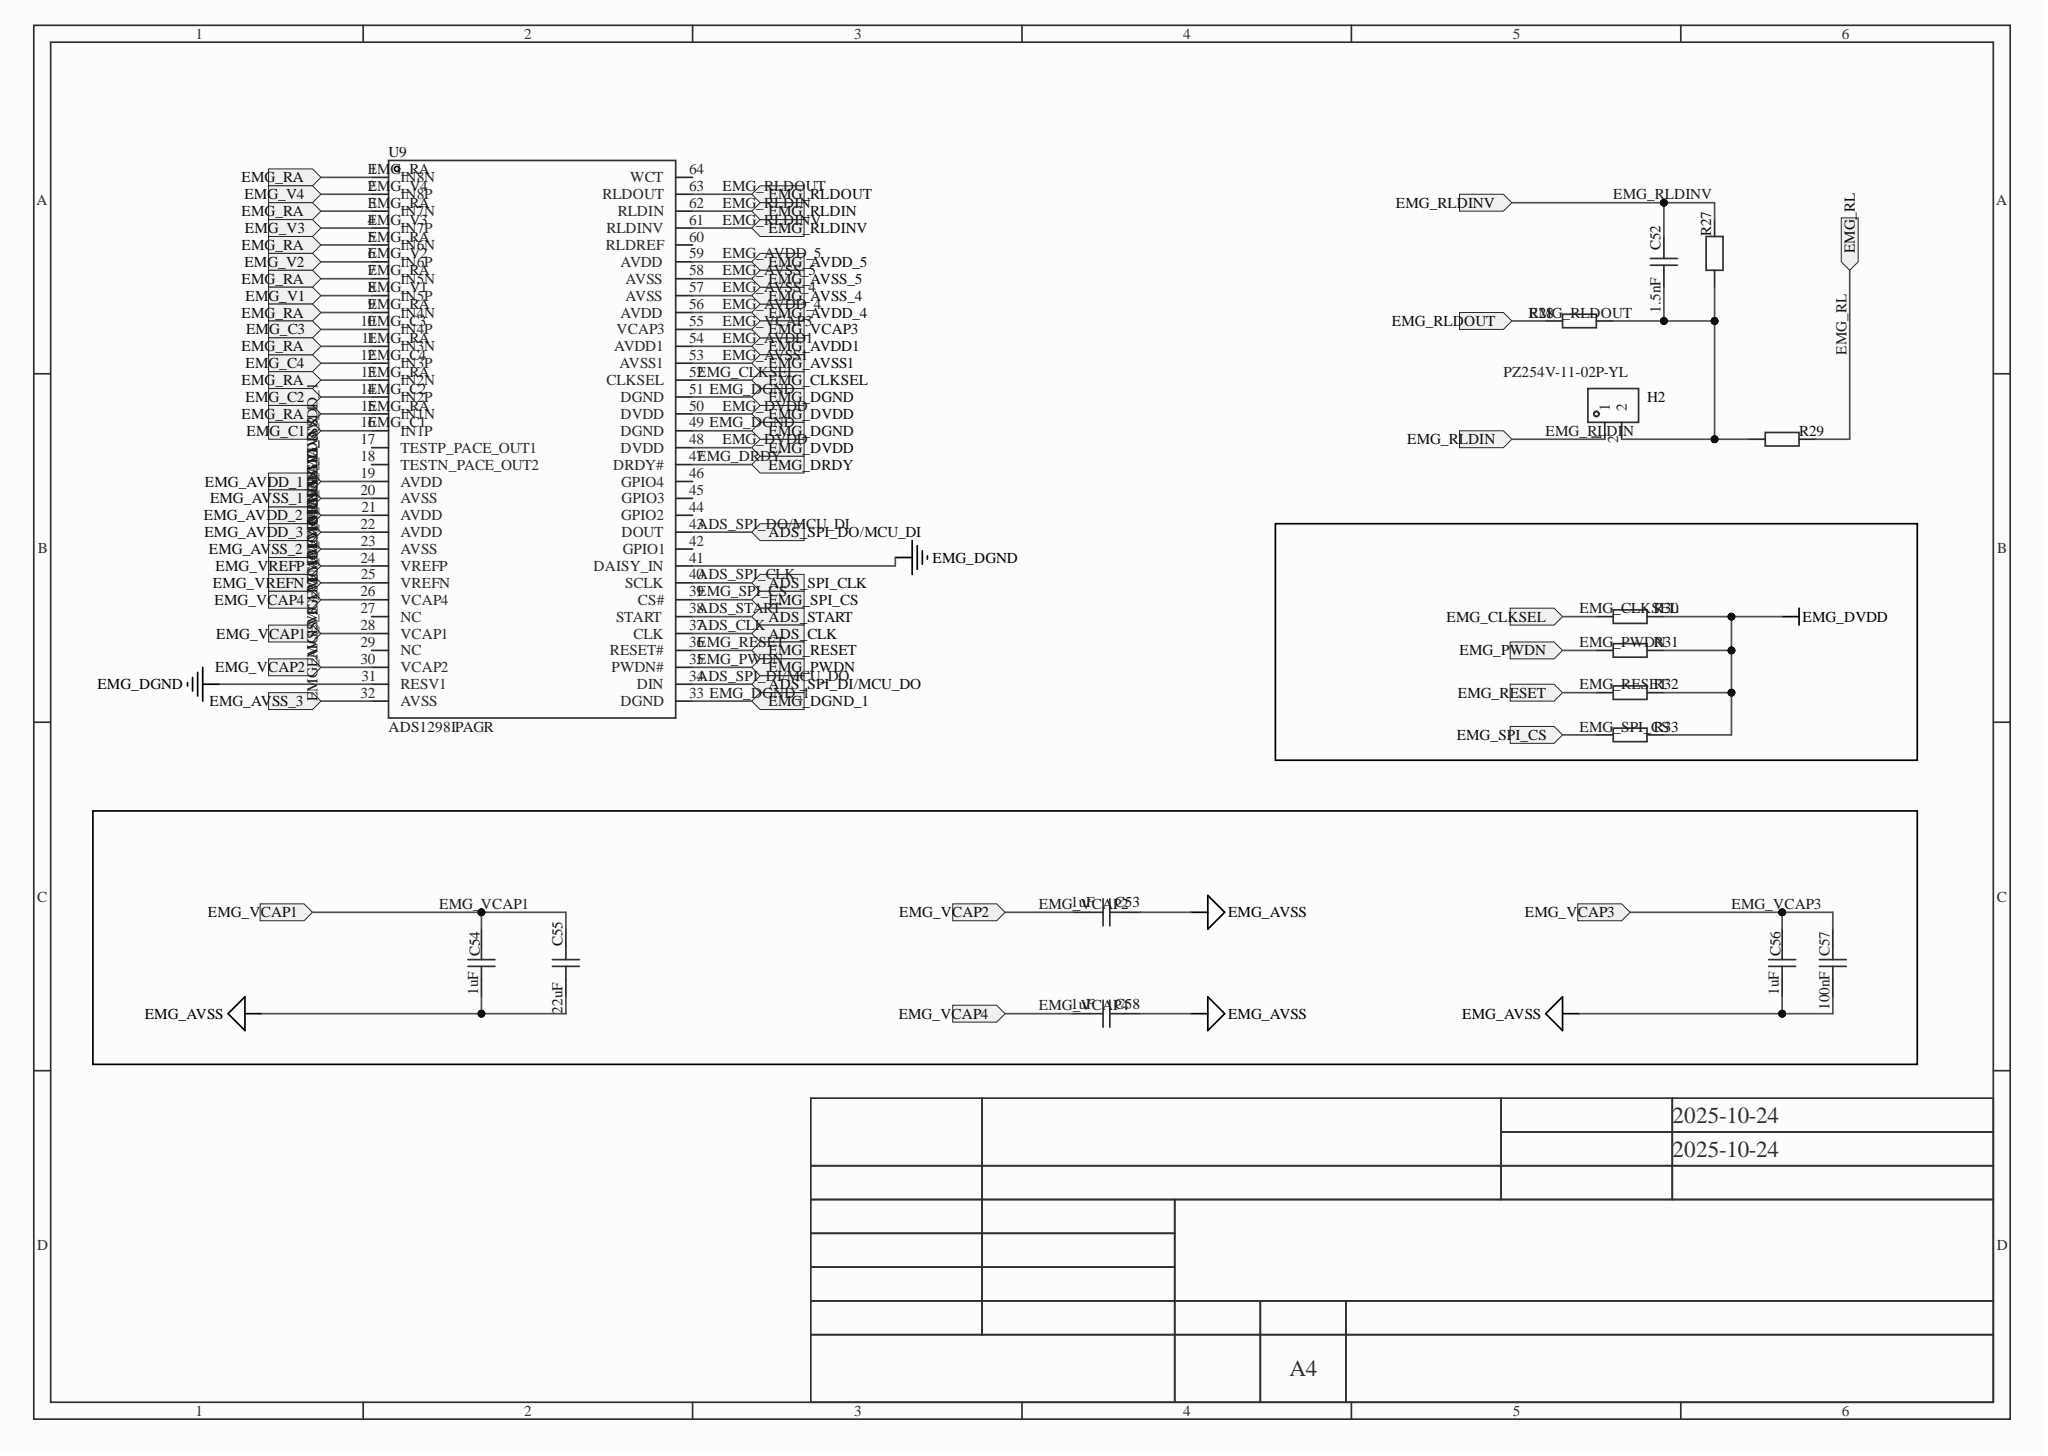Circuit board | Altium Designer | 212 parts | 123 nets | one sheet of the schematic
Parts on this sheet (reference | value | footprint):
C52 | 1.5nF | C0402
C53 | 1uF | C0402
C54 | 1uF | C0402
C55 | 22uF | C1206
C56 | 1uF | C0402
C57 | 100nF | C0402
C58 | 1uF | C0402
H2 | PZ254V-11-02P-YL | HDR-TH_2P-P2.54-V-M
R27 | R0402
R28 | R0402
R29 | R0402
R30 | R0402
R31 | R0402
R32 | R0402
R33 | R0402
U9 | ADS1298IPAGR | TQFP-64_L10.0-W10.0-P0.50-LS12.0-BL
Nets of these parts (net: part-pin ...):
NetC52_1: C52-1 H2-2 R27-2 R28-2 R29-1
EMG_VREFP: U9-24
EMG_VCAP4: C58-1 U9-26
EMG_VCAP3: C56-2 C57-2 U9-55
EMG_VCAP2: C53-1 U9-30
EMG_VCAP1: C54-2 C55-2 U9-28
EMG_V4: U9-2
EMG_V3: U9-4
EMG_V2: U9-6
EMG_V1: U9-8
EMG_SPI_CS: R33-1 U9-39
EMG_RLDOUT: R28-1 U9-63
EMG_RLDINV: C52-2 R27-1 U9-61
EMG_RLDIN: H2-1 U9-62
EMG_RL: R29-2
EMG_RESET: R32-1 U9-36
EMG_RA: U9-1 U9-3 U9-5 U9-7 U9-9 U9-11 U9-13 U9-15
EMG_PWDN: R31-1 U9-35
EMG_DVDD: R30-2 R31-2 R32-2 R33-2 U9-48 U9-50
EMG_DRDY: U9-47
EMG_DGND: U9-31 U9-33 U9-41 U9-49 U9-51
EMG_CLKSEL: R30-1 U9-52
EMG_C4: U9-12
EMG_C3: U9-10
EMG_C2: U9-14
EMG_C1: U9-16
EMG_AVSS1: C53-2 C54-1 C55-1 C56-1 C57-1 C58-2 U9-20 U9-23 U9-25 U9-32 U9-53 U9-57 U9-58
EMG_AVDD1: U9-19 U9-21 U9-22 U9-54 U9-56 U9-59
ADS_START: U9-38
ADS_SPI_DO/MCU_DI: U9-43
ADS_SPI_DI/MCU_DO: U9-34
ADS_SPI_CLK: U9-40
ADS_CLK: U9-37